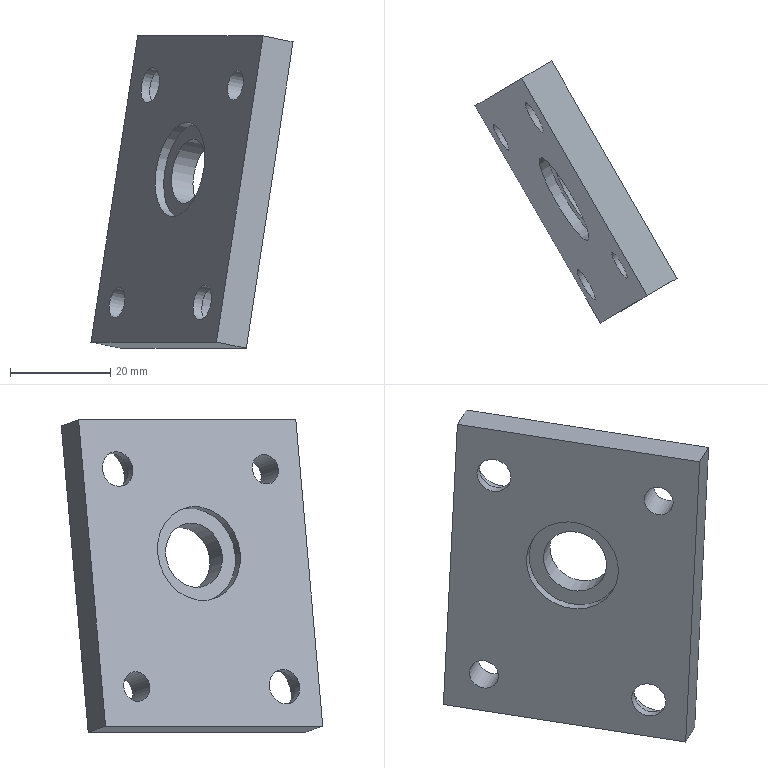Part | NX | features solid 2 | 1 solid | 17 faces | box 40.291 x 52.131 x 62.269 mm | volume 18965 mm3 | plane 9 | cylinder 8 | commonest cylinder face diameters 6 x2 7 x2 11 x2 13 x1 19 x1
STEP:
#1=CARTESIAN_POINT('',(-871.231,123.82,-53.981));
#2=VERTEX_POINT('',#1);
#3=CARTESIAN_POINT('',(-875.981,132.047,-53.981));
#4=DIRECTION('',(-0.8529,-0.4924,0.1736));
#5=DIRECTION('',(0.5,-0.866,0.));
#6=AXIS2_PLACEMENT_3D('',#3,#4,#5);
#7=CIRCLE('',#6,9.5);
#8=EDGE_CURVE('',#2,#2,#7,.T.);
#9=ORIENTED_EDGE('',*,*,#8,.F.);
#10=EDGE_LOOP('',(#9));
#11=FACE_BOUND('',#10,.T.);
#12=CARTESIAN_POINT('',(-873.282,118.017,-80.508));
#13=VERTEX_POINT('',#12);
#14=CARTESIAN_POINT('',(-871.532,114.986,-80.508));
#15=DIRECTION('',(0.8529,0.4924,-0.1736));
#16=DIRECTION('',(-0.5,0.866,0.));
#17=AXIS2_PLACEMENT_3D('',#14,#15,#16);
#18=CIRCLE('',#17,3.5);
#19=EDGE_CURVE('',#13,#13,#18,.T.);
#20=ORIENTED_EDGE('',*,*,#19,.T.);
#21=EDGE_LOOP('',(#20));
#22=FACE_BOUND('',#21,.T.);
#23=CARTESIAN_POINT('',(-890.032,147.029,-80.508));
#24=VERTEX_POINT('',#23);
#25=CARTESIAN_POINT('',(-888.532,144.431,-80.508));
#26=DIRECTION('',(0.8529,0.4924,-0.1736));
#27=DIRECTION('',(-0.5,0.866,0.));
#28=AXIS2_PLACEMENT_3D('',#25,#26,#27);
#29=CIRCLE('',#28,3.);
#30=EDGE_CURVE('',#24,#24,#29,.T.);
#31=ORIENTED_EDGE('',*,*,#30,.T.);
#32=EDGE_LOOP('',(#31));
#33=FACE_BOUND('',#32,.T.);
#34=CARTESIAN_POINT('',(-866.416,121.404,-37.18));
#35=VERTEX_POINT('',#34);
#36=CARTESIAN_POINT('',(-864.916,118.806,-37.18));
#37=DIRECTION('',(0.8529,0.4924,-0.1736));
#38=DIRECTION('',(-0.5,0.866,0.));
#39=AXIS2_PLACEMENT_3D('',#36,#37,#38);
#40=CIRCLE('',#39,3.);
#41=EDGE_CURVE('',#35,#35,#40,.T.);
#42=ORIENTED_EDGE('',*,*,#41,.T.);
#43=EDGE_LOOP('',(#42));
#44=FACE_BOUND('',#43,.T.);
#45=CARTESIAN_POINT('',(-883.664,151.282,-37.171));
#46=VERTEX_POINT('',#45);
#47=CARTESIAN_POINT('',(-881.914,148.251,-37.171));
#48=DIRECTION('',(0.8529,0.4924,-0.1736));
#49=DIRECTION('',(-0.5,0.866,0.));
#50=AXIS2_PLACEMENT_3D('',#47,#48,#49);
#51=CIRCLE('',#50,3.5);
#52=EDGE_CURVE('',#46,#46,#51,.T.);
#53=ORIENTED_EDGE('',*,*,#52,.T.);
#54=EDGE_LOOP('',(#53));
#55=FACE_BOUND('',#54,.T.);
#56=CARTESIAN_POINT('',(-893.735,150.664,-88.386));
#57=VERTEX_POINT('',#56);
#58=CARTESIAN_POINT('',(-868.735,107.363,-88.386));
#59=VERTEX_POINT('',#58);
#60=CARTESIAN_POINT('',(-909.778,178.451,-88.386));
#61=DIRECTION('',(0.5,-0.866,0.));
#62=VECTOR('',#61,1000.);
#63=LINE('',#60,#62);
#64=EDGE_CURVE('',#57,#59,#63,.T.);
#65=ORIENTED_EDGE('',*,*,#64,.T.);
#66=CARTESIAN_POINT('',(-859.414,112.744,-27.346));
#67=VERTEX_POINT('',#66);
#68=CARTESIAN_POINT('',(-864.975,109.534,-63.766));
#69=DIRECTION('',(0.1504,0.08682,0.9848));
#70=VECTOR('',#69,1000.);
#71=LINE('',#68,#70);
#72=EDGE_CURVE('',#59,#67,#71,.T.);
#73=ORIENTED_EDGE('',*,*,#72,.T.);
#74=CARTESIAN_POINT('',(-884.412,156.047,-27.333));
#75=VERTEX_POINT('',#74);
#76=CARTESIAN_POINT('',(-902.909,188.088,-27.323));
#77=DIRECTION('',(0.5,-0.866,-0.0002605));
#78=VECTOR('',#77,1000.);
#79=LINE('',#76,#78);
#80=EDGE_CURVE('',#75,#67,#79,.T.);
#81=ORIENTED_EDGE('',*,*,#80,.F.);
#82=CARTESIAN_POINT('',(-889.975,152.835,-63.766));
#83=DIRECTION('',(0.1504,0.08682,0.9848));
#84=VECTOR('',#83,1000.);
#85=LINE('',#82,#84);
#86=EDGE_CURVE('',#57,#75,#85,.T.);
#87=ORIENTED_EDGE('',*,*,#86,.F.);
#88=EDGE_LOOP('',(#65,#73,#81,#87));
#89=FACE_BOUND('',#88,.T.);
#90=CARTESIAN_POINT('',(-877.475,131.184,-63.766));
#91=DIRECTION('',(-0.8529,-0.4924,0.1736));
#92=DIRECTION('',(0.1504,0.08682,0.9848));
#93=AXIS2_PLACEMENT_3D('',#90,#91,#92);
#94=PLANE('',#93);
#95=ADVANCED_FACE('',(#11,#22,#33,#44,#55,#89),#94,.T.);
#96=ORIENTED_EDGE('',*,*,#80,.T.);
#97=CARTESIAN_POINT('',(-853.444,116.191,-28.561));
#98=VERTEX_POINT('',#97);
#99=CARTESIAN_POINT('',(-903.984,87.012,-18.271));
#100=DIRECTION('',(0.8529,0.4924,-0.1736));
#101=VECTOR('',#100,1000.);
#102=LINE('',#99,#101);
#103=EDGE_CURVE('',#67,#98,#102,.T.);
#104=ORIENTED_EDGE('',*,*,#103,.T.);
#105=CARTESIAN_POINT('',(-878.442,159.494,-28.548));
#106=VERTEX_POINT('',#105);
#107=CARTESIAN_POINT('',(-819.709,57.754,-28.579));
#108=DIRECTION('',(-0.5,0.866,0.0002605));
#109=VECTOR('',#108,1000.);
#110=LINE('',#107,#109);
#111=EDGE_CURVE('',#106,#98,#110,.F.);
#112=ORIENTED_EDGE('',*,*,#111,.F.);
#113=CARTESIAN_POINT('',(-928.982,130.314,-18.258));
#114=DIRECTION('',(0.8529,0.4924,-0.1736));
#115=VECTOR('',#114,1000.);
#116=LINE('',#113,#115);
#117=EDGE_CURVE('',#75,#106,#116,.T.);
#118=ORIENTED_EDGE('',*,*,#117,.F.);
#119=EDGE_LOOP('',(#96,#104,#112,#118));
#120=FACE_BOUND('',#119,.T.);
#121=CARTESIAN_POINT('',(-947.479,162.356,-18.248));
#122=DIRECTION('',(0.1505,0.08659,0.9848));
#123=DIRECTION('',(-0.8544,-0.4898,0.1736));
#124=AXIS2_PLACEMENT_3D('',#121,#122,#123);
#125=PLANE('',#124);
#126=ADVANCED_FACE('',(#120),#125,.T.);
#127=CARTESIAN_POINT('',(-866.761,129.865,-55.197));
#128=VERTEX_POINT('',#127);
#129=CARTESIAN_POINT('',(-870.011,135.494,-55.197));
#130=DIRECTION('',(-0.8529,-0.4924,0.1736));
#131=DIRECTION('',(0.5,-0.866,0.));
#132=AXIS2_PLACEMENT_3D('',#129,#130,#131);
#133=CIRCLE('',#132,6.5);
#134=EDGE_CURVE('',#128,#128,#133,.T.);
#135=ORIENTED_EDGE('',*,*,#134,.T.);
#136=EDGE_LOOP('',(#135));
#137=FACE_BOUND('',#136,.T.);
#138=CARTESIAN_POINT('',(-868.312,123.196,-81.723));
#139=VERTEX_POINT('',#138);
#140=CARTESIAN_POINT('',(-865.562,118.433,-81.723));
#141=DIRECTION('',(0.8529,0.4924,-0.1736));
#142=DIRECTION('',(-0.5,0.866,0.));
#143=AXIS2_PLACEMENT_3D('',#140,#141,#142);
#144=CIRCLE('',#143,5.5);
#145=EDGE_CURVE('',#139,#139,#144,.T.);
#146=ORIENTED_EDGE('',*,*,#145,.F.);
#147=EDGE_LOOP('',(#146));
#148=FACE_BOUND('',#147,.T.);
#149=CARTESIAN_POINT('',(-884.062,150.476,-81.723));
#150=VERTEX_POINT('',#149);
#151=CARTESIAN_POINT('',(-882.562,147.877,-81.723));
#152=DIRECTION('',(0.8529,0.4924,-0.1736));
#153=DIRECTION('',(-0.5,0.866,0.));
#154=AXIS2_PLACEMENT_3D('',#151,#152,#153);
#155=CIRCLE('',#154,3.);
#156=EDGE_CURVE('',#150,#150,#155,.T.);
#157=ORIENTED_EDGE('',*,*,#156,.F.);
#158=EDGE_LOOP('',(#157));
#159=FACE_BOUND('',#158,.T.);
#160=CARTESIAN_POINT('',(-860.446,124.851,-38.396));
#161=VERTEX_POINT('',#160);
#162=CARTESIAN_POINT('',(-858.946,122.252,-38.396));
#163=DIRECTION('',(0.8529,0.4924,-0.1736));
#164=DIRECTION('',(-0.5,0.866,0.));
#165=AXIS2_PLACEMENT_3D('',#162,#163,#164);
#166=CIRCLE('',#165,3.);
#167=EDGE_CURVE('',#161,#161,#166,.T.);
#168=ORIENTED_EDGE('',*,*,#167,.F.);
#169=EDGE_LOOP('',(#168));
#170=FACE_BOUND('',#169,.T.);
#171=CARTESIAN_POINT('',(-878.694,156.461,-38.387));
#172=VERTEX_POINT('',#171);
#173=CARTESIAN_POINT('',(-875.944,151.698,-38.387));
#174=DIRECTION('',(0.8529,0.4924,-0.1736));
#175=DIRECTION('',(-0.5,0.866,0.));
#176=AXIS2_PLACEMENT_3D('',#173,#174,#175);
#177=CIRCLE('',#176,5.5);
#178=EDGE_CURVE('',#172,#172,#177,.T.);
#179=ORIENTED_EDGE('',*,*,#178,.F.);
#180=EDGE_LOOP('',(#179));
#181=FACE_BOUND('',#180,.T.);
#182=ORIENTED_EDGE('',*,*,#111,.T.);
#183=CARTESIAN_POINT('',(-862.765,110.81,-89.602));
#184=VERTEX_POINT('',#183);
#185=CARTESIAN_POINT('',(-839.455,124.268,63.044));
#186=DIRECTION('',(-0.1504,-0.08682,-0.9848));
#187=VECTOR('',#186,1000.);
#188=LINE('',#185,#187);
#189=EDGE_CURVE('',#184,#98,#188,.F.);
#190=ORIENTED_EDGE('',*,*,#189,.F.);
#191=CARTESIAN_POINT('',(-887.765,154.111,-89.602));
#192=VERTEX_POINT('',#191);
#193=CARTESIAN_POINT('',(-829.015,52.353,-89.602));
#194=DIRECTION('',(-0.5,0.866,0.));
#195=VECTOR('',#194,1000.);
#196=LINE('',#193,#195);
#197=EDGE_CURVE('',#192,#184,#196,.F.);
#198=ORIENTED_EDGE('',*,*,#197,.F.);
#199=CARTESIAN_POINT('',(-864.455,167.569,63.044));
#200=DIRECTION('',(-0.1504,-0.08682,-0.9848));
#201=VECTOR('',#200,1000.);
#202=LINE('',#199,#201);
#203=EDGE_CURVE('',#192,#106,#202,.F.);
#204=ORIENTED_EDGE('',*,*,#203,.T.);
#205=EDGE_LOOP('',(#182,#190,#198,#204));
#206=FACE_BOUND('',#205,.T.);
#207=CARTESIAN_POINT('',(-805.705,65.811,63.044));
#208=DIRECTION('',(-0.8529,-0.4924,0.1736));
#209=DIRECTION('',(0.1504,0.08682,0.9848));
#210=AXIS2_PLACEMENT_3D('',#207,#208,#209);
#211=PLANE('',#210);
#212=ADVANCED_FACE('',(#137,#148,#159,#170,#181,#206),#211,.F.);
#213=CARTESIAN_POINT('',(-1066.867,50.706,-53.135));
#214=DIRECTION('',(0.8529,0.4924,-0.1736));
#215=VECTOR('',#214,1000.);
#216=LINE('',#213,#215);
#217=EDGE_CURVE('',#57,#192,#216,.T.);
#218=ORIENTED_EDGE('',*,*,#217,.T.);
#219=ORIENTED_EDGE('',*,*,#197,.T.);
#220=CARTESIAN_POINT('',(-1041.867,7.405,-53.135));
#221=DIRECTION('',(0.8529,0.4924,-0.1736));
#222=VECTOR('',#221,1000.);
#223=LINE('',#220,#222);
#224=EDGE_CURVE('',#59,#184,#223,.T.);
#225=ORIENTED_EDGE('',*,*,#224,.F.);
#226=ORIENTED_EDGE('',*,*,#64,.F.);
#227=EDGE_LOOP('',(#218,#219,#225,#226));
#228=FACE_BOUND('',#227,.T.);
#229=CARTESIAN_POINT('',(-1082.91,78.493,-53.135));
#230=DIRECTION('',(0.1504,0.08682,0.9848));
#231=DIRECTION('',(0.5,-0.866,0.));
#232=AXIS2_PLACEMENT_3D('',#229,#230,#231);
#233=PLANE('',#232);
#234=ADVANCED_FACE('',(#228),#233,.F.);
#235=ORIENTED_EDGE('',*,*,#189,.T.);
#236=ORIENTED_EDGE('',*,*,#103,.F.);
#237=ORIENTED_EDGE('',*,*,#72,.F.);
#238=ORIENTED_EDGE('',*,*,#224,.T.);
#239=EDGE_LOOP('',(#235,#236,#237,#238));
#240=FACE_BOUND('',#239,.T.);
#241=CARTESIAN_POINT('',(-864.975,109.534,-63.766));
#242=DIRECTION('',(0.5,-0.866,0.));
#243=DIRECTION('',(-0.8627,-0.4981,0.08716));
#244=AXIS2_PLACEMENT_3D('',#241,#242,#243);
#245=PLANE('',#244);
#246=ADVANCED_FACE('',(#240),#245,.T.);
#247=ORIENTED_EDGE('',*,*,#203,.F.);
#248=ORIENTED_EDGE('',*,*,#217,.F.);
#249=ORIENTED_EDGE('',*,*,#86,.T.);
#250=ORIENTED_EDGE('',*,*,#117,.T.);
#251=EDGE_LOOP('',(#247,#248,#249,#250));
#252=FACE_BOUND('',#251,.T.);
#253=CARTESIAN_POINT('',(-889.975,152.835,-63.766));
#254=DIRECTION('',(0.5,-0.866,0.));
#255=DIRECTION('',(-0.8627,-0.4981,0.08716));
#256=AXIS2_PLACEMENT_3D('',#253,#254,#255);
#257=PLANE('',#256);
#258=ADVANCED_FACE('',(#252),#257,.F.);
#259=ORIENTED_EDGE('',*,*,#52,.F.);
#260=EDGE_LOOP('',(#259));
#261=FACE_BOUND('',#260,.T.);
#262=CARTESIAN_POINT('',(-881.959,152.267,-37.519));
#263=VERTEX_POINT('',#262);
#264=CARTESIAN_POINT('',(-880.209,149.236,-37.519));
#265=DIRECTION('',(0.8529,0.4924,-0.1736));
#266=DIRECTION('',(-0.5,0.866,0.));
#267=AXIS2_PLACEMENT_3D('',#264,#265,#266);
#268=CIRCLE('',#267,3.5);
#269=EDGE_CURVE('',#263,#263,#268,.T.);
#270=ORIENTED_EDGE('',*,*,#269,.T.);
#271=EDGE_LOOP('',(#270));
#272=FACE_BOUND('',#271,.T.);
#273=CARTESIAN_POINT('',(-918.588,127.078,-29.705));
#274=DIRECTION('',(-0.8529,-0.4924,0.1736));
#275=DIRECTION('',(-0.5,0.866,0.));
#276=AXIS2_PLACEMENT_3D('',#273,#274,#275);
#277=CYLINDRICAL_SURFACE('',#276,3.5);
#278=ADVANCED_FACE('',(#261,#272),#277,.F.);
#279=ORIENTED_EDGE('',*,*,#269,.F.);
#280=EDGE_LOOP('',(#279));
#281=FACE_BOUND('',#280,.T.);
#282=CARTESIAN_POINT('',(-882.959,153.999,-37.519));
#283=VERTEX_POINT('',#282);
#284=CARTESIAN_POINT('',(-880.209,149.236,-37.519));
#285=DIRECTION('',(0.8529,0.4924,-0.1736));
#286=DIRECTION('',(-0.5,0.866,0.));
#287=AXIS2_PLACEMENT_3D('',#284,#285,#286);
#288=CIRCLE('',#287,5.5);
#289=EDGE_CURVE('',#283,#283,#288,.T.);
#290=ORIENTED_EDGE('',*,*,#289,.T.);
#291=EDGE_LOOP('',(#290));
#292=FACE_BOUND('',#291,.T.);
#293=CARTESIAN_POINT('',(-881.712,148.368,-47.367));
#294=DIRECTION('',(-0.8529,-0.4924,0.1736));
#295=DIRECTION('',(-0.5,0.866,0.));
#296=AXIS2_PLACEMENT_3D('',#293,#294,#295);
#297=PLANE('',#296);
#298=ADVANCED_FACE('',(#281,#292),#297,.F.);
#299=ORIENTED_EDGE('',*,*,#289,.F.);
#300=EDGE_LOOP('',(#299));
#301=FACE_BOUND('',#300,.T.);
#302=ORIENTED_EDGE('',*,*,#178,.T.);
#303=EDGE_LOOP('',(#302));
#304=FACE_BOUND('',#303,.T.);
#305=CARTESIAN_POINT('',(-875.944,151.698,-38.387));
#306=DIRECTION('',(-0.8529,-0.4924,0.1736));
#307=DIRECTION('',(-0.5,0.866,0.));
#308=AXIS2_PLACEMENT_3D('',#305,#306,#307);
#309=CYLINDRICAL_SURFACE('',#308,5.5);
#310=ADVANCED_FACE('',(#301,#304),#309,.F.);
#311=ORIENTED_EDGE('',*,*,#41,.F.);
#312=EDGE_LOOP('',(#311));
#313=FACE_BOUND('',#312,.T.);
#314=ORIENTED_EDGE('',*,*,#167,.T.);
#315=EDGE_LOOP('',(#314));
#316=FACE_BOUND('',#315,.T.);
#317=CARTESIAN_POINT('',(-901.589,97.632,-29.713));
#318=DIRECTION('',(-0.8529,-0.4924,0.1736));
#319=DIRECTION('',(-0.5,0.866,0.));
#320=AXIS2_PLACEMENT_3D('',#317,#318,#319);
#321=CYLINDRICAL_SURFACE('',#320,3.);
#322=ADVANCED_FACE('',(#313,#316),#321,.F.);
#323=ORIENTED_EDGE('',*,*,#30,.F.);
#324=EDGE_LOOP('',(#323));
#325=FACE_BOUND('',#324,.T.);
#326=ORIENTED_EDGE('',*,*,#156,.T.);
#327=EDGE_LOOP('',(#326));
#328=FACE_BOUND('',#327,.T.);
#329=CARTESIAN_POINT('',(-925.205,123.257,-73.041));
#330=DIRECTION('',(-0.8529,-0.4924,0.1736));
#331=DIRECTION('',(-0.5,0.866,0.));
#332=AXIS2_PLACEMENT_3D('',#329,#330,#331);
#333=CYLINDRICAL_SURFACE('',#332,3.);
#334=ADVANCED_FACE('',(#325,#328),#333,.F.);
#335=ORIENTED_EDGE('',*,*,#19,.F.);
#336=EDGE_LOOP('',(#335));
#337=FACE_BOUND('',#336,.T.);
#338=CARTESIAN_POINT('',(-871.576,119.002,-80.855));
#339=VERTEX_POINT('',#338);
#340=CARTESIAN_POINT('',(-869.826,115.971,-80.855));
#341=DIRECTION('',(0.8529,0.4924,-0.1736));
#342=DIRECTION('',(-0.5,0.866,0.));
#343=AXIS2_PLACEMENT_3D('',#340,#341,#342);
#344=CIRCLE('',#343,3.5);
#345=EDGE_CURVE('',#339,#339,#344,.T.);
#346=ORIENTED_EDGE('',*,*,#345,.T.);
#347=EDGE_LOOP('',(#346));
#348=FACE_BOUND('',#347,.T.);
#349=CARTESIAN_POINT('',(-908.205,93.812,-73.041));
#350=DIRECTION('',(-0.8529,-0.4924,0.1736));
#351=DIRECTION('',(-0.5,0.866,0.));
#352=AXIS2_PLACEMENT_3D('',#349,#350,#351);
#353=CYLINDRICAL_SURFACE('',#352,3.5);
#354=ADVANCED_FACE('',(#337,#348),#353,.F.);
#355=ORIENTED_EDGE('',*,*,#345,.F.);
#356=EDGE_LOOP('',(#355));
#357=FACE_BOUND('',#356,.T.);
#358=CARTESIAN_POINT('',(-872.576,120.734,-80.855));
#359=VERTEX_POINT('',#358);
#360=CARTESIAN_POINT('',(-869.826,115.971,-80.855));
#361=DIRECTION('',(0.8529,0.4924,-0.1736));
#362=DIRECTION('',(-0.5,0.866,0.));
#363=AXIS2_PLACEMENT_3D('',#360,#361,#362);
#364=CIRCLE('',#363,5.5);
#365=EDGE_CURVE('',#359,#359,#364,.T.);
#366=ORIENTED_EDGE('',*,*,#365,.T.);
#367=EDGE_LOOP('',(#366));
#368=FACE_BOUND('',#367,.T.);
#369=CARTESIAN_POINT('',(-871.33,115.102,-90.703));
#370=DIRECTION('',(-0.8529,-0.4924,0.1736));
#371=DIRECTION('',(-0.5,0.866,0.));
#372=AXIS2_PLACEMENT_3D('',#369,#370,#371);
#373=PLANE('',#372);
#374=ADVANCED_FACE('',(#357,#368),#373,.F.);
#375=ORIENTED_EDGE('',*,*,#365,.F.);
#376=EDGE_LOOP('',(#375));
#377=FACE_BOUND('',#376,.T.);
#378=ORIENTED_EDGE('',*,*,#145,.T.);
#379=EDGE_LOOP('',(#378));
#380=FACE_BOUND('',#379,.T.);
#381=CARTESIAN_POINT('',(-865.562,118.433,-81.723));
#382=DIRECTION('',(-0.8529,-0.4924,0.1736));
#383=DIRECTION('',(-0.5,0.866,0.));
#384=AXIS2_PLACEMENT_3D('',#381,#382,#383);
#385=CYLINDRICAL_SURFACE('',#384,5.5);
#386=ADVANCED_FACE('',(#377,#380),#385,.F.);
#387=CARTESIAN_POINT('',(-877.525,138.661,-54.328));
#388=VERTEX_POINT('',#387);
#389=CARTESIAN_POINT('',(-874.275,133.032,-54.328));
#390=DIRECTION('',(0.8529,0.4924,-0.1736));
#391=DIRECTION('',(-0.5,0.866,0.));
#392=AXIS2_PLACEMENT_3D('',#389,#390,#391);
#393=CIRCLE('',#392,6.5);
#394=EDGE_CURVE('',#388,#388,#393,.F.);
#395=ORIENTED_EDGE('',*,*,#394,.T.);
#396=EDGE_LOOP('',(#395));
#397=FACE_BOUND('',#396,.T.);
#398=ORIENTED_EDGE('',*,*,#134,.F.);
#399=EDGE_LOOP('',(#398));
#400=FACE_BOUND('',#399,.T.);
#401=CARTESIAN_POINT('',(-872.57,134.016,-54.676));
#402=DIRECTION('',(0.8529,0.4924,-0.1736));
#403=DIRECTION('',(0.2933,-0.727,-0.6209));
#404=AXIS2_PLACEMENT_3D('',#401,#402,#403);
#405=CYLINDRICAL_SURFACE('',#404,6.5);
#406=ADVANCED_FACE('',(#397,#400),#405,.F.);
#407=ORIENTED_EDGE('',*,*,#394,.F.);
#408=EDGE_LOOP('',(#407));
#409=FACE_BOUND('',#408,.T.);
#410=CARTESIAN_POINT('',(-879.025,141.259,-54.328));
#411=VERTEX_POINT('',#410);
#412=CARTESIAN_POINT('',(-874.275,133.032,-54.328));
#413=DIRECTION('',(0.8529,0.4924,-0.1736));
#414=DIRECTION('',(-0.5,0.866,0.));
#415=AXIS2_PLACEMENT_3D('',#412,#413,#414);
#416=CIRCLE('',#415,9.5);
#417=EDGE_CURVE('',#411,#411,#416,.T.);
#418=ORIENTED_EDGE('',*,*,#417,.F.);
#419=EDGE_LOOP('',(#418));
#420=FACE_BOUND('',#419,.T.);
#421=CARTESIAN_POINT('',(-874.275,133.032,-54.328));
#422=DIRECTION('',(0.8529,0.4924,-0.1736));
#423=DIRECTION('',(0.2933,-0.727,-0.6209));
#424=AXIS2_PLACEMENT_3D('',#421,#422,#423);
#425=PLANE('',#424);
#426=ADVANCED_FACE('',(#409,#420),#425,.F.);
#427=ORIENTED_EDGE('',*,*,#8,.T.);
#428=EDGE_LOOP('',(#427));
#429=FACE_BOUND('',#428,.T.);
#430=ORIENTED_EDGE('',*,*,#417,.T.);
#431=EDGE_LOOP('',(#430));
#432=FACE_BOUND('',#431,.T.);
#433=CARTESIAN_POINT('',(-957.857,84.776,-37.311));
#434=DIRECTION('',(0.8529,0.4924,-0.1736));
#435=DIRECTION('',(0.2933,-0.727,-0.6209));
#436=AXIS2_PLACEMENT_3D('',#433,#434,#435);
#437=CYLINDRICAL_SURFACE('',#436,9.5);
#438=ADVANCED_FACE('',(#429,#432),#437,.F.);
#439=CLOSED_SHELL('',(#95,#126,#212,#234,#246,#258,#278,#298,#310,#322,#334,#354,#374,#386,#406,#426,#438));
#440=MANIFOLD_SOLID_BREP('',#439);
#441=(LENGTH_UNIT()NAMED_UNIT(*)SI_UNIT(.MILLI.,.METRE.));
#442=UNCERTAINTY_MEASURE_WITH_UNIT(LENGTH_MEASURE(0.00001),#441,'','');
#443=(NAMED_UNIT(*)PLANE_ANGLE_UNIT()SI_UNIT($,.RADIAN.));
#444=(NAMED_UNIT(*)SI_UNIT($,.STERADIAN.)SOLID_ANGLE_UNIT());
#445=(GEOMETRIC_REPRESENTATION_CONTEXT(3)GLOBAL_UNCERTAINTY_ASSIGNED_CONTEXT((#442))GLOBAL_UNIT_ASSIGNED_CONTEXT((#441,#443,#444))REPRESENTATION_CONTEXT('',''));
#446=ADVANCED_BREP_SHAPE_REPRESENTATION('',(#440),#445);